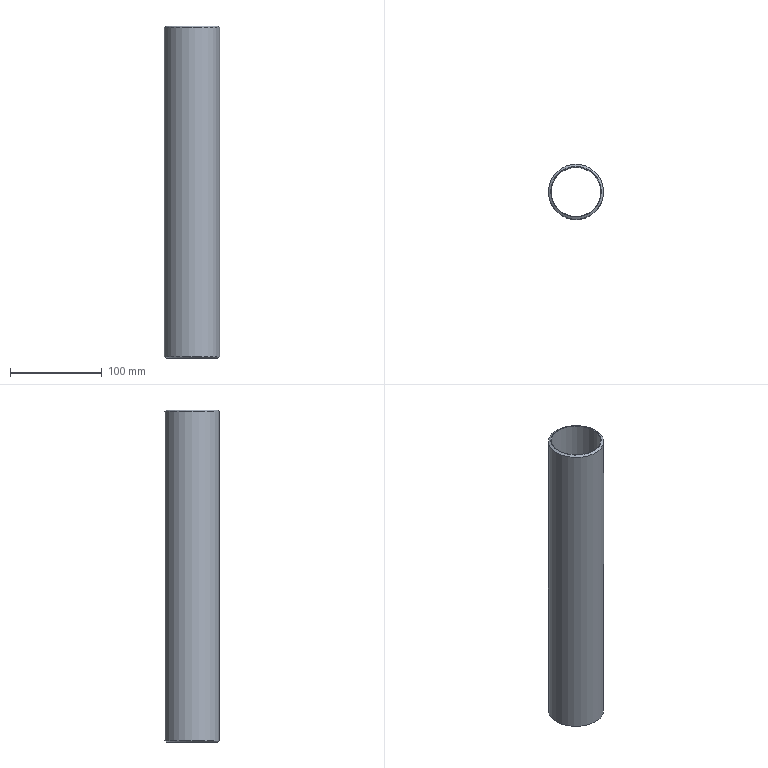Part | NX | features CHAMFER 2, CYLINDER 1, DATUM_CSYS 1, SHELL 1 | 1 solid | 6 faces | box 60 x 60 x 361 mm | volume 193272 mm3 | plane 2 | cylinder 2 | cone 2 | commonest cylinder face diameters 54 x1 60 x1
STEP:
#1=CARTESIAN_POINT('',(27.5,0.,361.));
#2=VERTEX_POINT('',#1);
#3=CARTESIAN_POINT('',(0.,0.,361.));
#4=DIRECTION('',(0.,0.,1.));
#5=DIRECTION('',(1.,0.,0.));
#6=AXIS2_PLACEMENT_3D('',#3,#4,#5);
#7=CIRCLE('',#6,27.5);
#8=EDGE_CURVE('',#2,#2,#7,.T.);
#9=ORIENTED_EDGE('',*,*,#8,.T.);
#10=EDGE_LOOP('',(#9));
#11=FACE_BOUND('',#10,.T.);
#12=CARTESIAN_POINT('',(27.,0.,361.));
#13=VERTEX_POINT('',#12);
#14=CARTESIAN_POINT('',(0.,0.,361.));
#15=DIRECTION('',(0.,0.,1.));
#16=DIRECTION('',(1.,0.,0.));
#17=AXIS2_PLACEMENT_3D('',#14,#15,#16);
#18=CIRCLE('',#17,27.);
#19=EDGE_CURVE('',#13,#13,#18,.F.);
#20=ORIENTED_EDGE('',*,*,#19,.T.);
#21=EDGE_LOOP('',(#20));
#22=FACE_BOUND('',#21,.T.);
#23=CARTESIAN_POINT('',(0.,0.,361.));
#24=DIRECTION('',(0.,0.,1.));
#25=DIRECTION('',(1.,0.,0.));
#26=AXIS2_PLACEMENT_3D('',#23,#24,#25);
#27=PLANE('',#26);
#28=ADVANCED_FACE('',(#11,#22),#27,.T.);
#29=CARTESIAN_POINT('',(-27.5,0.,0.));
#30=VERTEX_POINT('',#29);
#31=CARTESIAN_POINT('',(0.,0.,0.));
#32=DIRECTION('',(0.,0.,-1.));
#33=DIRECTION('',(-1.,0.,0.));
#34=AXIS2_PLACEMENT_3D('',#31,#32,#33);
#35=CIRCLE('',#34,27.5);
#36=EDGE_CURVE('',#30,#30,#35,.T.);
#37=ORIENTED_EDGE('',*,*,#36,.T.);
#38=EDGE_LOOP('',(#37));
#39=FACE_BOUND('',#38,.T.);
#40=CARTESIAN_POINT('',(-27.,0.,0.));
#41=VERTEX_POINT('',#40);
#42=CARTESIAN_POINT('',(0.,0.,0.));
#43=DIRECTION('',(0.,0.,-1.));
#44=DIRECTION('',(-1.,0.,0.));
#45=AXIS2_PLACEMENT_3D('',#42,#43,#44);
#46=CIRCLE('',#45,27.);
#47=EDGE_CURVE('',#41,#41,#46,.F.);
#48=ORIENTED_EDGE('',*,*,#47,.T.);
#49=EDGE_LOOP('',(#48));
#50=FACE_BOUND('',#49,.T.);
#51=CARTESIAN_POINT('',(0.,0.,0.));
#52=DIRECTION('',(0.,0.,-1.));
#53=DIRECTION('',(-1.,0.,0.));
#54=AXIS2_PLACEMENT_3D('',#51,#52,#53);
#55=PLANE('',#54);
#56=ADVANCED_FACE('',(#39,#50),#55,.T.);
#57=CARTESIAN_POINT('',(30.,0.,359.557));
#58=VERTEX_POINT('',#57);
#59=CARTESIAN_POINT('',(0.,0.,359.557));
#60=DIRECTION('',(0.,0.,1.));
#61=DIRECTION('',(1.,0.,0.));
#62=AXIS2_PLACEMENT_3D('',#59,#60,#61);
#63=CIRCLE('',#62,30.);
#64=EDGE_CURVE('',#58,#58,#63,.F.);
#65=ORIENTED_EDGE('',*,*,#64,.T.);
#66=EDGE_LOOP('',(#65));
#67=FACE_BOUND('',#66,.T.);
#68=CARTESIAN_POINT('',(-30.,0.,1.443));
#69=VERTEX_POINT('',#68);
#70=CARTESIAN_POINT('',(0.,0.,1.443));
#71=DIRECTION('',(0.,0.,-1.));
#72=DIRECTION('',(-1.,0.,0.));
#73=AXIS2_PLACEMENT_3D('',#70,#71,#72);
#74=CIRCLE('',#73,30.);
#75=EDGE_CURVE('',#69,#69,#74,.F.);
#76=ORIENTED_EDGE('',*,*,#75,.T.);
#77=EDGE_LOOP('',(#76));
#78=FACE_BOUND('',#77,.T.);
#79=CARTESIAN_POINT('',(0.,0.,0.));
#80=DIRECTION('',(0.,0.,1.));
#81=DIRECTION('',(1.,0.,0.));
#82=AXIS2_PLACEMENT_3D('',#79,#80,#81);
#83=CYLINDRICAL_SURFACE('',#82,30.);
#84=ADVANCED_FACE('',(#67,#78),#83,.T.);
#85=ORIENTED_EDGE('',*,*,#19,.F.);
#86=EDGE_LOOP('',(#85));
#87=FACE_BOUND('',#86,.T.);
#88=ORIENTED_EDGE('',*,*,#47,.F.);
#89=EDGE_LOOP('',(#88));
#90=FACE_BOUND('',#89,.T.);
#91=CARTESIAN_POINT('',(0.,0.,0.));
#92=DIRECTION('',(0.,0.,1.));
#93=DIRECTION('',(1.,0.,0.));
#94=AXIS2_PLACEMENT_3D('',#91,#92,#93);
#95=CYLINDRICAL_SURFACE('',#94,27.);
#96=ADVANCED_FACE('',(#87,#90),#95,.F.);
#97=ORIENTED_EDGE('',*,*,#36,.F.);
#98=EDGE_LOOP('',(#97));
#99=FACE_BOUND('',#98,.T.);
#100=ORIENTED_EDGE('',*,*,#75,.F.);
#101=EDGE_LOOP('',(#100));
#102=FACE_BOUND('',#101,.T.);
#103=CARTESIAN_POINT('',(0.,0.,1.443));
#104=DIRECTION('',(0.,0.,1.));
#105=DIRECTION('',(1.,0.,0.));
#106=AXIS2_PLACEMENT_3D('',#103,#104,#105);
#107=CONICAL_SURFACE('',#106,30.,1.047);
#108=ADVANCED_FACE('',(#99,#102),#107,.T.);
#109=ORIENTED_EDGE('',*,*,#8,.F.);
#110=EDGE_LOOP('',(#109));
#111=FACE_BOUND('',#110,.T.);
#112=ORIENTED_EDGE('',*,*,#64,.F.);
#113=EDGE_LOOP('',(#112));
#114=FACE_BOUND('',#113,.T.);
#115=CARTESIAN_POINT('',(0.,0.,359.557));
#116=DIRECTION('',(0.,0.,-1.));
#117=DIRECTION('',(-1.,0.,0.));
#118=AXIS2_PLACEMENT_3D('',#115,#116,#117);
#119=CONICAL_SURFACE('',#118,30.,1.047);
#120=ADVANCED_FACE('',(#111,#114),#119,.T.);
#121=CLOSED_SHELL('',(#28,#56,#84,#96,#108,#120));
#122=MANIFOLD_SOLID_BREP('',#121);
#123=(LENGTH_UNIT()NAMED_UNIT(*)SI_UNIT(.MILLI.,.METRE.));
#124=UNCERTAINTY_MEASURE_WITH_UNIT(LENGTH_MEASURE(0.00001),#123,'','');
#125=(NAMED_UNIT(*)PLANE_ANGLE_UNIT()SI_UNIT($,.RADIAN.));
#126=(NAMED_UNIT(*)SI_UNIT($,.STERADIAN.)SOLID_ANGLE_UNIT());
#127=(GEOMETRIC_REPRESENTATION_CONTEXT(3)GLOBAL_UNCERTAINTY_ASSIGNED_CONTEXT((#124))GLOBAL_UNIT_ASSIGNED_CONTEXT((#123,#125,#126))REPRESENTATION_CONTEXT('',''));
#128=ADVANCED_BREP_SHAPE_REPRESENTATION('',(#122),#127);